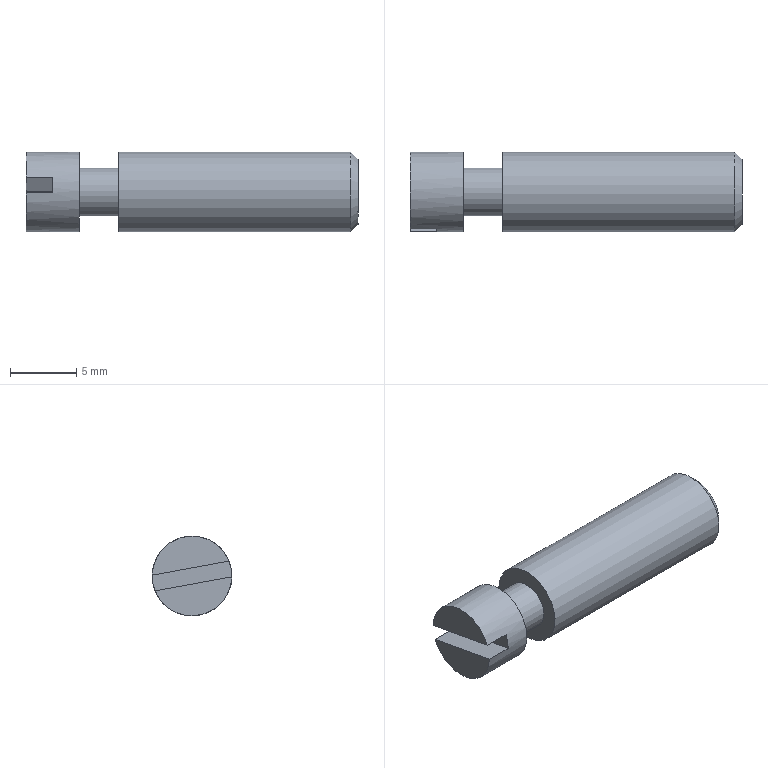Part | NX | features 1 2 | 1 solid | 12 faces | box 25 x 6 x 6 mm | volume 635.671 mm3 | plane 8 | cylinder 3 | cone 1 | commonest cylinder face diameters 6 x2 3.6 x1
STEP:
#1=CARTESIAN_POINT('',(-6.242,51.055,-650.874));
#2=VERTEX_POINT('',#1);
#3=CARTESIAN_POINT('',(-6.242,51.593,-647.922));
#4=DIRECTION('',(-1.,0.,0.));
#5=DIRECTION('',(0.,-0.1793,-0.9838));
#6=AXIS2_PLACEMENT_3D('',#3,#4,#5);
#7=CIRCLE('',#6,3.);
#8=EDGE_CURVE('',#2,#2,#7,.T.);
#9=ORIENTED_EDGE('',*,*,#8,.T.);
#10=EDGE_LOOP('',(#9));
#11=FACE_BOUND('',#10,.T.);
#12=CARTESIAN_POINT('',(-23.7,51.055,-650.874));
#13=VERTEX_POINT('',#12);
#14=CARTESIAN_POINT('',(-23.7,51.593,-647.922));
#15=DIRECTION('',(1.,0.,0.));
#16=DIRECTION('',(0.,-0.1793,-0.9838));
#17=AXIS2_PLACEMENT_3D('',#14,#15,#16);
#18=CIRCLE('',#17,3.);
#19=EDGE_CURVE('',#13,#13,#18,.T.);
#20=ORIENTED_EDGE('',*,*,#19,.T.);
#21=EDGE_LOOP('',(#20));
#22=FACE_BOUND('',#21,.T.);
#23=CARTESIAN_POINT('',(-18.471,51.593,-647.922));
#24=DIRECTION('',(1.,0.,0.));
#25=DIRECTION('',(0.,0.1793,0.9838));
#26=AXIS2_PLACEMENT_3D('',#23,#24,#25);
#27=CYLINDRICAL_SURFACE('',#26,3.);
#28=ADVANCED_FACE('',(#11,#22),#27,.T.);
#29=ORIENTED_EDGE('',*,*,#8,.F.);
#30=EDGE_LOOP('',(#29));
#31=FACE_BOUND('',#30,.T.);
#32=CARTESIAN_POINT('',(-5.7,52.034,-645.504));
#33=VERTEX_POINT('',#32);
#34=CARTESIAN_POINT('',(-5.7,51.593,-647.922));
#35=DIRECTION('',(-1.,0.,0.));
#36=DIRECTION('',(0.,0.1793,0.9838));
#37=AXIS2_PLACEMENT_3D('',#34,#35,#36);
#38=CIRCLE('',#37,2.459);
#39=EDGE_CURVE('',#33,#33,#38,.T.);
#40=ORIENTED_EDGE('',*,*,#39,.T.);
#41=EDGE_LOOP('',(#40));
#42=FACE_BOUND('',#41,.T.);
#43=CARTESIAN_POINT('',(-6.242,51.593,-647.922));
#44=DIRECTION('',(-1.,0.,0.));
#45=DIRECTION('',(0.,-0.1793,-0.9838));
#46=AXIS2_PLACEMENT_3D('',#43,#44,#45);
#47=CONICAL_SURFACE('',#46,3.,0.7854);
#48=ADVANCED_FACE('',(#31,#42),#47,.T.);
#49=CARTESIAN_POINT('',(-23.7,51.271,-649.693));
#50=VERTEX_POINT('',#49);
#51=CARTESIAN_POINT('',(-23.7,51.593,-647.922));
#52=DIRECTION('',(-1.,0.,0.));
#53=DIRECTION('',(0.,-0.1793,-0.9838));
#54=AXIS2_PLACEMENT_3D('',#51,#52,#53);
#55=CIRCLE('',#54,1.8);
#56=EDGE_CURVE('',#50,#50,#55,.T.);
#57=ORIENTED_EDGE('',*,*,#56,.T.);
#58=EDGE_LOOP('',(#57));
#59=FACE_BOUND('',#58,.T.);
#60=CARTESIAN_POINT('',(-26.7,51.271,-649.693));
#61=VERTEX_POINT('',#60);
#62=CARTESIAN_POINT('',(-26.7,51.593,-647.922));
#63=DIRECTION('',(1.,0.,0.));
#64=DIRECTION('',(0.,-0.1793,-0.9838));
#65=AXIS2_PLACEMENT_3D('',#62,#63,#64);
#66=CIRCLE('',#65,1.8);
#67=EDGE_CURVE('',#61,#61,#66,.T.);
#68=ORIENTED_EDGE('',*,*,#67,.T.);
#69=EDGE_LOOP('',(#68));
#70=FACE_BOUND('',#69,.T.);
#71=CARTESIAN_POINT('',(-25.2,51.593,-647.922));
#72=DIRECTION('',(1.,0.,0.));
#73=DIRECTION('',(0.,0.1793,0.9838));
#74=AXIS2_PLACEMENT_3D('',#71,#72,#73);
#75=CYLINDRICAL_SURFACE('',#74,1.8);
#76=ADVANCED_FACE('',(#59,#70),#75,.T.);
#77=CARTESIAN_POINT('',(-26.7,51.055,-650.874));
#78=VERTEX_POINT('',#77);
#79=CARTESIAN_POINT('',(-26.7,51.593,-647.922));
#80=DIRECTION('',(-1.,0.,0.));
#81=DIRECTION('',(0.,-0.1793,-0.9838));
#82=AXIS2_PLACEMENT_3D('',#79,#80,#81);
#83=CIRCLE('',#82,3.);
#84=EDGE_CURVE('',#78,#78,#83,.T.);
#85=ORIENTED_EDGE('',*,*,#84,.T.);
#86=EDGE_LOOP('',(#85));
#87=FACE_BOUND('',#86,.T.);
#88=CARTESIAN_POINT('',(-30.7,54.593,-647.859));
#89=VERTEX_POINT('',#88);
#90=CARTESIAN_POINT('',(-30.7,48.809,-646.805));
#91=VERTEX_POINT('',#90);
#92=CARTESIAN_POINT('',(-30.7,51.593,-647.922));
#93=DIRECTION('',(1.,0.,0.));
#94=DIRECTION('',(0.,-0.1793,-0.9838));
#95=AXIS2_PLACEMENT_3D('',#92,#93,#94);
#96=CIRCLE('',#95,3.);
#97=EDGE_CURVE('',#89,#91,#96,.T.);
#98=ORIENTED_EDGE('',*,*,#97,.T.);
#99=CARTESIAN_POINT('',(-28.7,48.809,-646.805));
#100=VERTEX_POINT('',#99);
#101=CARTESIAN_POINT('',(-18.471,48.809,-646.805));
#102=DIRECTION('',(1.,0.,0.));
#103=VECTOR('',#102,1000.);
#104=LINE('',#101,#103);
#105=EDGE_CURVE('',#91,#100,#104,.T.);
#106=ORIENTED_EDGE('',*,*,#105,.T.);
#107=CARTESIAN_POINT('',(-28.7,48.594,-647.986));
#108=VERTEX_POINT('',#107);
#109=CARTESIAN_POINT('',(-28.7,51.593,-647.922));
#110=DIRECTION('',(1.,0.,0.));
#111=DIRECTION('',(0.,-0.1793,-0.9838));
#112=AXIS2_PLACEMENT_3D('',#109,#110,#111);
#113=CIRCLE('',#112,3.);
#114=EDGE_CURVE('',#100,#108,#113,.T.);
#115=ORIENTED_EDGE('',*,*,#114,.T.);
#116=CARTESIAN_POINT('',(-30.7,48.594,-647.986));
#117=VERTEX_POINT('',#116);
#118=CARTESIAN_POINT('',(-18.471,48.594,-647.986));
#119=DIRECTION('',(-1.,0.,0.));
#120=VECTOR('',#119,1000.);
#121=LINE('',#118,#120);
#122=EDGE_CURVE('',#108,#117,#121,.T.);
#123=ORIENTED_EDGE('',*,*,#122,.T.);
#124=CARTESIAN_POINT('',(-30.7,54.377,-649.039));
#125=VERTEX_POINT('',#124);
#126=CARTESIAN_POINT('',(-30.7,51.593,-647.922));
#127=DIRECTION('',(1.,0.,0.));
#128=DIRECTION('',(0.,-0.1793,-0.9838));
#129=AXIS2_PLACEMENT_3D('',#126,#127,#128);
#130=CIRCLE('',#129,3.);
#131=EDGE_CURVE('',#117,#125,#130,.T.);
#132=ORIENTED_EDGE('',*,*,#131,.T.);
#133=CARTESIAN_POINT('',(-28.7,54.377,-649.039));
#134=VERTEX_POINT('',#133);
#135=CARTESIAN_POINT('',(-18.471,54.377,-649.039));
#136=DIRECTION('',(1.,0.,0.));
#137=VECTOR('',#136,1000.);
#138=LINE('',#135,#137);
#139=EDGE_CURVE('',#125,#134,#138,.T.);
#140=ORIENTED_EDGE('',*,*,#139,.T.);
#141=CARTESIAN_POINT('',(-28.7,54.593,-647.859));
#142=VERTEX_POINT('',#141);
#143=CARTESIAN_POINT('',(-28.7,51.593,-647.922));
#144=DIRECTION('',(1.,0.,0.));
#145=DIRECTION('',(0.,-0.1793,-0.9838));
#146=AXIS2_PLACEMENT_3D('',#143,#144,#145);
#147=CIRCLE('',#146,3.);
#148=EDGE_CURVE('',#134,#142,#147,.T.);
#149=ORIENTED_EDGE('',*,*,#148,.T.);
#150=CARTESIAN_POINT('',(-18.471,54.593,-647.859));
#151=DIRECTION('',(-1.,0.,0.));
#152=VECTOR('',#151,1000.);
#153=LINE('',#150,#152);
#154=EDGE_CURVE('',#142,#89,#153,.T.);
#155=ORIENTED_EDGE('',*,*,#154,.T.);
#156=EDGE_LOOP('',(#98,#106,#115,#123,#132,#140,#149,#155));
#157=FACE_BOUND('',#156,.T.);
#158=CARTESIAN_POINT('',(-18.471,51.593,-647.922));
#159=DIRECTION('',(1.,0.,0.));
#160=DIRECTION('',(0.,0.1793,0.9838));
#161=AXIS2_PLACEMENT_3D('',#158,#159,#160);
#162=CYLINDRICAL_SURFACE('',#161,3.);
#163=ADVANCED_FACE('',(#87,#157),#162,.T.);
#164=ORIENTED_EDGE('',*,*,#56,.F.);
#165=EDGE_LOOP('',(#164));
#166=FACE_BOUND('',#165,.T.);
#167=ORIENTED_EDGE('',*,*,#19,.F.);
#168=EDGE_LOOP('',(#167));
#169=FACE_BOUND('',#168,.T.);
#170=CARTESIAN_POINT('',(-23.7,54.84,-648.514));
#171=DIRECTION('',(1.,0.,0.));
#172=DIRECTION('',(0.,0.1793,0.9838));
#173=AXIS2_PLACEMENT_3D('',#170,#171,#172);
#174=PLANE('',#173);
#175=ADVANCED_FACE('',(#166,#169),#174,.F.);
#176=ORIENTED_EDGE('',*,*,#39,.F.);
#177=EDGE_LOOP('',(#176));
#178=FACE_BOUND('',#177,.T.);
#179=CARTESIAN_POINT('',(-5.7,52.803,-648.143));
#180=DIRECTION('',(1.,0.,0.));
#181=DIRECTION('',(0.,0.1793,0.9838));
#182=AXIS2_PLACEMENT_3D('',#179,#180,#181);
#183=PLANE('',#182);
#184=ADVANCED_FACE('',(#178),#183,.T.);
#185=ORIENTED_EDGE('',*,*,#67,.F.);
#186=EDGE_LOOP('',(#185));
#187=FACE_BOUND('',#186,.T.);
#188=ORIENTED_EDGE('',*,*,#84,.F.);
#189=EDGE_LOOP('',(#188));
#190=FACE_BOUND('',#189,.T.);
#191=CARTESIAN_POINT('',(-26.7,54.84,-648.514));
#192=DIRECTION('',(-1.,0.,0.));
#193=DIRECTION('',(0.,-0.1793,-0.9838));
#194=AXIS2_PLACEMENT_3D('',#191,#192,#193);
#195=PLANE('',#194);
#196=ADVANCED_FACE('',(#187,#190),#195,.F.);
#197=CARTESIAN_POINT('',(-30.7,54.652,-647.87));
#198=DIRECTION('',(0.,-0.9838,0.1793));
#199=VECTOR('',#198,1000.);
#200=LINE('',#197,#199);
#201=EDGE_CURVE('',#89,#91,#200,.T.);
#202=ORIENTED_EDGE('',*,*,#201,.F.);
#203=ORIENTED_EDGE('',*,*,#154,.F.);
#204=CARTESIAN_POINT('',(-28.7,54.652,-647.87));
#205=DIRECTION('',(0.,0.9838,-0.1793));
#206=VECTOR('',#205,1000.);
#207=LINE('',#204,#206);
#208=EDGE_CURVE('',#100,#142,#207,.T.);
#209=ORIENTED_EDGE('',*,*,#208,.F.);
#210=ORIENTED_EDGE('',*,*,#105,.F.);
#211=EDGE_LOOP('',(#202,#203,#209,#210));
#212=FACE_BOUND('',#211,.T.);
#213=CARTESIAN_POINT('',(-30.7,54.652,-647.87));
#214=DIRECTION('',(0.,0.1793,0.9838));
#215=DIRECTION('',(-1.,0.,0.));
#216=AXIS2_PLACEMENT_3D('',#213,#214,#215);
#217=PLANE('',#216);
#218=ADVANCED_FACE('',(#212),#217,.F.);
#219=ORIENTED_EDGE('',*,*,#201,.T.);
#220=ORIENTED_EDGE('',*,*,#97,.F.);
#221=EDGE_LOOP('',(#219,#220));
#222=FACE_BOUND('',#221,.T.);
#223=CARTESIAN_POINT('',(-30.7,53.069,-648.191));
#224=DIRECTION('',(-1.,0.,0.));
#225=DIRECTION('',(0.,-0.1793,-0.9838));
#226=AXIS2_PLACEMENT_3D('',#223,#224,#225);
#227=PLANE('',#226);
#228=ADVANCED_FACE('',(#222),#227,.T.);
#229=CARTESIAN_POINT('',(-28.7,54.437,-649.05));
#230=DIRECTION('',(0.,-0.9838,0.1793));
#231=VECTOR('',#230,1000.);
#232=LINE('',#229,#231);
#233=EDGE_CURVE('',#134,#108,#232,.T.);
#234=ORIENTED_EDGE('',*,*,#233,.F.);
#235=ORIENTED_EDGE('',*,*,#139,.F.);
#236=CARTESIAN_POINT('',(-30.7,54.437,-649.05));
#237=DIRECTION('',(0.,0.9838,-0.1793));
#238=VECTOR('',#237,1000.);
#239=LINE('',#236,#238);
#240=EDGE_CURVE('',#117,#125,#239,.T.);
#241=ORIENTED_EDGE('',*,*,#240,.F.);
#242=ORIENTED_EDGE('',*,*,#122,.F.);
#243=EDGE_LOOP('',(#234,#235,#241,#242));
#244=FACE_BOUND('',#243,.T.);
#245=CARTESIAN_POINT('',(-28.7,54.437,-649.05));
#246=DIRECTION('',(0.,-0.1793,-0.9838));
#247=DIRECTION('',(1.,0.,0.));
#248=AXIS2_PLACEMENT_3D('',#245,#246,#247);
#249=PLANE('',#248);
#250=ADVANCED_FACE('',(#244),#249,.F.);
#251=ORIENTED_EDGE('',*,*,#240,.T.);
#252=ORIENTED_EDGE('',*,*,#131,.F.);
#253=EDGE_LOOP('',(#251,#252));
#254=FACE_BOUND('',#253,.T.);
#255=CARTESIAN_POINT('',(-30.7,53.069,-648.191));
#256=DIRECTION('',(-1.,0.,0.));
#257=DIRECTION('',(0.,-0.1793,-0.9838));
#258=AXIS2_PLACEMENT_3D('',#255,#256,#257);
#259=PLANE('',#258);
#260=ADVANCED_FACE('',(#254),#259,.T.);
#261=ORIENTED_EDGE('',*,*,#208,.T.);
#262=ORIENTED_EDGE('',*,*,#148,.F.);
#263=ORIENTED_EDGE('',*,*,#233,.T.);
#264=ORIENTED_EDGE('',*,*,#114,.F.);
#265=EDGE_LOOP('',(#261,#262,#263,#264));
#266=FACE_BOUND('',#265,.T.);
#267=CARTESIAN_POINT('',(-28.7,54.652,-647.87));
#268=DIRECTION('',(1.,0.,0.));
#269=DIRECTION('',(0.,0.1793,0.9838));
#270=AXIS2_PLACEMENT_3D('',#267,#268,#269);
#271=PLANE('',#270);
#272=ADVANCED_FACE('',(#266),#271,.F.);
#273=CLOSED_SHELL('',(#28,#48,#76,#163,#175,#184,#196,#218,#228,#250,#260,#272));
#274=MANIFOLD_SOLID_BREP('',#273);
#275=(LENGTH_UNIT()NAMED_UNIT(*)SI_UNIT(.MILLI.,.METRE.));
#276=UNCERTAINTY_MEASURE_WITH_UNIT(LENGTH_MEASURE(0.00001),#275,'','');
#277=(NAMED_UNIT(*)PLANE_ANGLE_UNIT()SI_UNIT($,.RADIAN.));
#278=(NAMED_UNIT(*)SI_UNIT($,.STERADIAN.)SOLID_ANGLE_UNIT());
#279=(GEOMETRIC_REPRESENTATION_CONTEXT(3)GLOBAL_UNCERTAINTY_ASSIGNED_CONTEXT((#276))GLOBAL_UNIT_ASSIGNED_CONTEXT((#275,#277,#278))REPRESENTATION_CONTEXT('',''));
#280=ADVANCED_BREP_SHAPE_REPRESENTATION('',(#274),#279);